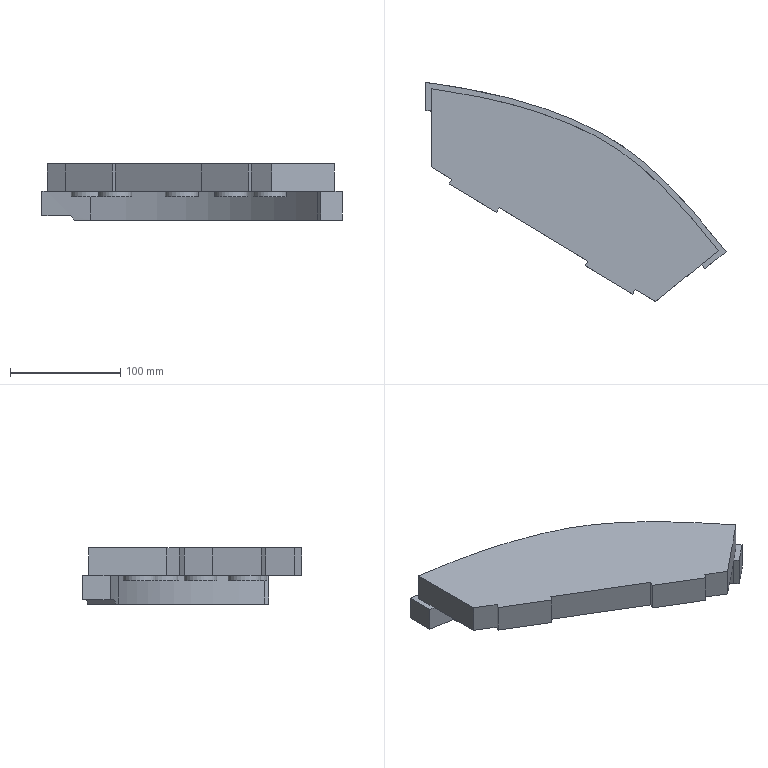Part | NX | features solid 2 | 1 solid | 36 faces | box 271.95 x 198.601 x 51 mm | volume 834371 mm3 | plane 25 | spline 6 | cylinder 5 | commonest cylinder face diameters 30 x5
STEP:
#1=CARTESIAN_POINT('',(-298.429,-300.345,20.));
#2=VERTEX_POINT('',#1);
#3=CARTESIAN_POINT('',(-283.429,-300.345,20.));
#4=DIRECTION('',(0.,0.,-1.));
#5=DIRECTION('',(-1.,0.,0.));
#6=AXIS2_PLACEMENT_3D('',#3,#4,#5);
#7=CIRCLE('',#6,15.);
#8=EDGE_CURVE('',#2,#2,#7,.T.);
#9=ORIENTED_EDGE('',*,*,#8,.F.);
#10=EDGE_LOOP('',(#9));
#11=FACE_BOUND('',#10,.T.);
#12=CARTESIAN_POINT('',(-213.429,-355.345,20.));
#13=VERTEX_POINT('',#12);
#14=CARTESIAN_POINT('',(-198.429,-355.345,20.));
#15=DIRECTION('',(0.,0.,-1.));
#16=DIRECTION('',(-1.,0.,0.));
#17=AXIS2_PLACEMENT_3D('',#14,#15,#16);
#18=CIRCLE('',#17,15.);
#19=EDGE_CURVE('',#13,#13,#18,.T.);
#20=ORIENTED_EDGE('',*,*,#19,.F.);
#21=EDGE_LOOP('',(#20));
#22=FACE_BOUND('',#21,.T.);
#23=CARTESIAN_POINT('',(-103.429,-400.345,20.));
#24=VERTEX_POINT('',#23);
#25=CARTESIAN_POINT('',(-118.429,-400.345,20.));
#26=DIRECTION('',(0.,0.,1.));
#27=DIRECTION('',(1.,0.,0.));
#28=AXIS2_PLACEMENT_3D('',#25,#26,#27);
#29=CIRCLE('',#28,15.);
#30=EDGE_CURVE('',#24,#24,#29,.T.);
#31=ORIENTED_EDGE('',*,*,#30,.T.);
#32=EDGE_LOOP('',(#31));
#33=FACE_BOUND('',#32,.T.);
#34=CARTESIAN_POINT('',(-320.,-324.952,20.));
#35=VERTEX_POINT('',#34);
#36=CARTESIAN_POINT('',(-320.,-274.295,20.));
#37=VERTEX_POINT('',#36);
#38=CARTESIAN_POINT('',(-320.,-348.688,20.));
#39=DIRECTION('',(0.,1.,0.));
#40=VECTOR('',#39,1000.);
#41=LINE('',#38,#40);
#42=EDGE_CURVE('',#35,#37,#41,.T.);
#43=ORIENTED_EDGE('',*,*,#42,.T.);
#44=CARTESIAN_POINT('',(-280.742,-281.088,20.));
#45=VERTEX_POINT('',#44);
#46=CARTESIAN_POINT('',(-280.742,-281.088,20.));
#47=CARTESIAN_POINT('',(-293.762,-278.446,20.));
#48=CARTESIAN_POINT('',(-306.859,-276.24,20.));
#49=CARTESIAN_POINT('',(-320.,-274.295,20.));
#50=B_SPLINE_CURVE_WITH_KNOTS('',3,(#46,#47,#48,#49),.UNSPECIFIED.,.F.,.F.,(4,4),(1.18,1.219),.UNSPECIFIED.);
#51=EDGE_CURVE('',#45,#37,#50,.T.);
#52=ORIENTED_EDGE('',*,*,#51,.F.);
#53=CARTESIAN_POINT('',(-280.742,-281.088,20.));
#54=VERTEX_POINT('',#53);
#55=CARTESIAN_POINT('',(-303.787,-389.506,20.));
#56=DIRECTION('',(-0.2079,-0.9781,0.));
#57=VECTOR('',#56,1000.);
#58=LINE('',#55,#57);
#59=EDGE_CURVE('',#45,#54,#58,.F.);
#60=ORIENTED_EDGE('',*,*,#59,.T.);
#61=CARTESIAN_POINT('',(-75.598,-413.386,20.));
#62=VERTEX_POINT('',#61);
#63=CARTESIAN_POINT('',(-280.742,-281.088,20.));
#64=CARTESIAN_POINT('',(-270.509,-283.168,20.));
#65=CARTESIAN_POINT('',(-250.227,-287.836,20.));
#66=CARTESIAN_POINT('',(-225.511,-295.448,20.));
#67=CARTESIAN_POINT('',(-206.19,-302.794,20.));
#68=CARTESIAN_POINT('',(-191.924,-308.939,20.));
#69=CARTESIAN_POINT('',(-177.971,-315.925,20.));
#70=CARTESIAN_POINT('',(-164.415,-324.129,20.));
#71=CARTESIAN_POINT('',(-151.409,-333.446,20.));
#72=CARTESIAN_POINT('',(-135.17,-346.814,20.));
#73=CARTESIAN_POINT('',(-116.381,-365.121,20.));
#74=CARTESIAN_POINT('',(-95.487,-388.742,20.));
#75=CARTESIAN_POINT('',(-82.188,-405.145,20.));
#76=CARTESIAN_POINT('',(-75.598,-413.386,20.));
#77=B_SPLINE_CURVE_WITH_KNOTS('',3,(#63,#64,#65,#66,#67,#68,#69,#70,#71,#72,#73,#74,#75,#76),.UNSPECIFIED.,.F.,.F.,(4,1,1,1,1,1,1,1,1,1,1,4),(0.9834,1.015,1.046,1.062,1.077,1.093,1.109,1.124,1.14,1.171,1.203,1.234),.UNSPECIFIED.);
#78=EDGE_CURVE('',#62,#54,#77,.F.);
#79=ORIENTED_EDGE('',*,*,#78,.F.);
#80=CARTESIAN_POINT('',(-117.01,-446.921,20.));
#81=VERTEX_POINT('',#80);
#82=CARTESIAN_POINT('',(-152.811,-475.913,20.));
#83=DIRECTION('',(0.7771,0.6293,0.));
#84=VECTOR('',#83,1000.);
#85=LINE('',#82,#84);
#86=EDGE_CURVE('',#81,#62,#85,.T.);
#87=ORIENTED_EDGE('',*,*,#86,.F.);
#88=CARTESIAN_POINT('',(-135.335,-435.91,20.));
#89=VERTEX_POINT('',#88);
#90=CARTESIAN_POINT('',(-344.41,-310.285,20.));
#91=DIRECTION('',(-0.8572,0.515,0.));
#92=VECTOR('',#91,1000.);
#93=LINE('',#90,#92);
#94=EDGE_CURVE('',#89,#81,#93,.F.);
#95=ORIENTED_EDGE('',*,*,#94,.F.);
#96=CARTESIAN_POINT('',(-137.91,-440.196,20.));
#97=VERTEX_POINT('',#96);
#98=CARTESIAN_POINT('',(-135.335,-435.91,20.));
#99=DIRECTION('',(-0.515,-0.8572,0.));
#100=VECTOR('',#99,1000.);
#101=LINE('',#98,#100);
#102=EDGE_CURVE('',#89,#97,#101,.T.);
#103=ORIENTED_EDGE('',*,*,#102,.T.);
#104=CARTESIAN_POINT('',(-180.768,-414.444,20.));
#105=VERTEX_POINT('',#104);
#106=CARTESIAN_POINT('',(-185.054,-411.869,20.));
#107=DIRECTION('',(0.8572,-0.515,0.));
#108=VECTOR('',#107,1000.);
#109=LINE('',#106,#108);
#110=EDGE_CURVE('',#105,#97,#109,.T.);
#111=ORIENTED_EDGE('',*,*,#110,.F.);
#112=CARTESIAN_POINT('',(-178.193,-410.158,20.));
#113=VERTEX_POINT('',#112);
#114=CARTESIAN_POINT('',(-178.193,-410.158,20.));
#115=DIRECTION('',(-0.515,-0.8572,0.));
#116=VECTOR('',#115,1000.);
#117=LINE('',#114,#116);
#118=EDGE_CURVE('',#113,#105,#117,.T.);
#119=ORIENTED_EDGE('',*,*,#118,.F.);
#120=CARTESIAN_POINT('',(-258.498,-361.906,20.));
#121=VERTEX_POINT('',#120);
#122=CARTESIAN_POINT('',(-344.41,-310.285,20.));
#123=DIRECTION('',(-0.8572,0.515,0.));
#124=VECTOR('',#123,1000.);
#125=LINE('',#122,#124);
#126=EDGE_CURVE('',#121,#113,#125,.F.);
#127=ORIENTED_EDGE('',*,*,#126,.F.);
#128=CARTESIAN_POINT('',(-261.073,-366.192,20.));
#129=VERTEX_POINT('',#128);
#130=CARTESIAN_POINT('',(-221.506,-300.342,20.));
#131=DIRECTION('',(0.515,0.8572,0.));
#132=VECTOR('',#131,1000.);
#133=LINE('',#130,#132);
#134=EDGE_CURVE('',#121,#129,#133,.F.);
#135=ORIENTED_EDGE('',*,*,#134,.T.);
#136=CARTESIAN_POINT('',(-303.932,-340.44,20.));
#137=VERTEX_POINT('',#136);
#138=CARTESIAN_POINT('',(-286.788,-350.741,20.));
#139=DIRECTION('',(0.8572,-0.515,0.));
#140=VECTOR('',#139,1000.);
#141=LINE('',#138,#140);
#142=EDGE_CURVE('',#137,#129,#141,.T.);
#143=ORIENTED_EDGE('',*,*,#142,.F.);
#144=CARTESIAN_POINT('',(-301.356,-336.154,20.));
#145=VERTEX_POINT('',#144);
#146=CARTESIAN_POINT('',(-264.365,-274.59,20.));
#147=DIRECTION('',(0.515,0.8572,0.));
#148=VECTOR('',#147,1000.);
#149=LINE('',#146,#148);
#150=EDGE_CURVE('',#145,#137,#149,.F.);
#151=ORIENTED_EDGE('',*,*,#150,.F.);
#152=CARTESIAN_POINT('',(-344.41,-310.285,20.));
#153=DIRECTION('',(-0.8572,0.515,0.));
#154=VECTOR('',#153,1000.);
#155=LINE('',#152,#154);
#156=EDGE_CURVE('',#35,#145,#155,.F.);
#157=ORIENTED_EDGE('',*,*,#156,.F.);
#158=EDGE_LOOP('',(#43,#52,#60,#79,#87,#95,#103,#111,#119,#127,#135,#143,#151,#157));
#159=FACE_BOUND('',#158,.T.);
#160=CARTESIAN_POINT('',(-273.429,-320.345,20.));
#161=VERTEX_POINT('',#160);
#162=CARTESIAN_POINT('',(-258.429,-320.345,20.));
#163=DIRECTION('',(0.,0.,-1.));
#164=DIRECTION('',(-1.,0.,0.));
#165=AXIS2_PLACEMENT_3D('',#162,#163,#164);
#166=CIRCLE('',#165,15.);
#167=EDGE_CURVE('',#161,#161,#166,.T.);
#168=ORIENTED_EDGE('',*,*,#167,.F.);
#169=EDGE_LOOP('',(#168));
#170=FACE_BOUND('',#169,.T.);
#171=CARTESIAN_POINT('',(-168.429,-395.345,20.));
#172=VERTEX_POINT('',#171);
#173=CARTESIAN_POINT('',(-153.429,-395.345,20.));
#174=DIRECTION('',(0.,0.,-1.));
#175=DIRECTION('',(-1.,0.,0.));
#176=AXIS2_PLACEMENT_3D('',#173,#174,#175);
#177=CIRCLE('',#176,15.);
#178=EDGE_CURVE('',#172,#172,#177,.T.);
#179=ORIENTED_EDGE('',*,*,#178,.F.);
#180=EDGE_LOOP('',(#179));
#181=FACE_BOUND('',#180,.T.);
#182=CARTESIAN_POINT('',(-53.05,-401.561,20.));
#183=DIRECTION('',(0.,0.,-1.));
#184=DIRECTION('',(-1.,0.,0.));
#185=AXIS2_PLACEMENT_3D('',#182,#183,#184);
#186=PLANE('',#185);
#187=ADVANCED_FACE('',(#11,#22,#33,#159,#170,#181),#186,.T.);
#188=CARTESIAN_POINT('',(-325.,-273.568,-2.));
#189=VERTEX_POINT('',#188);
#190=CARTESIAN_POINT('',(-325.,-248.32,-2.));
#191=VERTEX_POINT('',#190);
#192=CARTESIAN_POINT('',(-325.,-560.,-2.));
#193=DIRECTION('',(0.,1.,0.));
#194=VECTOR('',#193,1000.);
#195=LINE('',#192,#194);
#196=EDGE_CURVE('',#189,#191,#195,.T.);
#197=ORIENTED_EDGE('',*,*,#196,.F.);
#198=CARTESIAN_POINT('',(-325.,-273.568,20.));
#199=VERTEX_POINT('',#198);
#200=CARTESIAN_POINT('',(-325.,-273.568,7.));
#201=DIRECTION('',(0.,0.,1.));
#202=VECTOR('',#201,1000.);
#203=LINE('',#200,#202);
#204=EDGE_CURVE('',#199,#189,#203,.F.);
#205=ORIENTED_EDGE('',*,*,#204,.F.);
#206=CARTESIAN_POINT('',(-325.,-248.32,20.));
#207=VERTEX_POINT('',#206);
#208=CARTESIAN_POINT('',(-325.,-401.561,20.));
#209=DIRECTION('',(0.,1.,0.));
#210=VECTOR('',#209,1000.);
#211=LINE('',#208,#210);
#212=EDGE_CURVE('',#207,#199,#211,.F.);
#213=ORIENTED_EDGE('',*,*,#212,.F.);
#214=CARTESIAN_POINT('',(-325.,-248.32,7.));
#215=DIRECTION('',(0.,0.,-1.));
#216=VECTOR('',#215,1000.);
#217=LINE('',#214,#216);
#218=EDGE_CURVE('',#191,#207,#217,.F.);
#219=ORIENTED_EDGE('',*,*,#218,.F.);
#220=EDGE_LOOP('',(#197,#205,#213,#219));
#221=FACE_BOUND('',#220,.T.);
#222=CARTESIAN_POINT('',(-325.,-560.,0.));
#223=DIRECTION('',(1.,0.,0.));
#224=DIRECTION('',(0.,0.,-1.));
#225=AXIS2_PLACEMENT_3D('',#222,#223,#224);
#226=PLANE('',#225);
#227=ADVANCED_FACE('',(#221),#226,.F.);
#228=CARTESIAN_POINT('',(-320.,-324.952,45.));
#229=VERTEX_POINT('',#228);
#230=CARTESIAN_POINT('',(-320.,-324.952,70.));
#231=DIRECTION('',(0.,0.,1.));
#232=VECTOR('',#231,1000.);
#233=LINE('',#230,#232);
#234=EDGE_CURVE('',#35,#229,#233,.T.);
#235=ORIENTED_EDGE('',*,*,#234,.F.);
#236=ORIENTED_EDGE('',*,*,#156,.T.);
#237=CARTESIAN_POINT('',(-301.356,-336.154,45.));
#238=VERTEX_POINT('',#237);
#239=CARTESIAN_POINT('',(-301.356,-336.154,45.));
#240=DIRECTION('',(0.,0.,-1.));
#241=VECTOR('',#240,1000.);
#242=LINE('',#239,#241);
#243=EDGE_CURVE('',#238,#145,#242,.T.);
#244=ORIENTED_EDGE('',*,*,#243,.F.);
#245=CARTESIAN_POINT('',(-344.41,-310.285,45.));
#246=DIRECTION('',(0.8572,-0.515,0.));
#247=VECTOR('',#246,1000.);
#248=LINE('',#245,#247);
#249=EDGE_CURVE('',#229,#238,#248,.T.);
#250=ORIENTED_EDGE('',*,*,#249,.F.);
#251=EDGE_LOOP('',(#235,#236,#244,#250));
#252=FACE_BOUND('',#251,.T.);
#253=CARTESIAN_POINT('',(-344.41,-310.285,70.));
#254=DIRECTION('',(0.515,0.8572,0.));
#255=DIRECTION('',(-0.8572,0.515,0.));
#256=AXIS2_PLACEMENT_3D('',#253,#254,#255);
#257=PLANE('',#256);
#258=ADVANCED_FACE('',(#252),#257,.F.);
#259=CARTESIAN_POINT('',(-320.,-254.082,45.));
#260=VERTEX_POINT('',#259);
#261=CARTESIAN_POINT('',(-320.,-254.082,20.));
#262=VERTEX_POINT('',#261);
#263=CARTESIAN_POINT('',(-320.,-254.082,32.5));
#264=DIRECTION('',(0.,0.,-1.));
#265=VECTOR('',#264,1000.);
#266=LINE('',#263,#265);
#267=EDGE_CURVE('',#260,#262,#266,.T.);
#268=ORIENTED_EDGE('',*,*,#267,.F.);
#269=CARTESIAN_POINT('',(-276.584,-261.524,45.));
#270=VERTEX_POINT('',#269);
#271=CARTESIAN_POINT('',(-276.584,-261.524,45.));
#272=CARTESIAN_POINT('',(-290.986,-258.597,45.));
#273=CARTESIAN_POINT('',(-305.47,-256.189,45.));
#274=CARTESIAN_POINT('',(-320.,-254.082,45.));
#275=B_SPLINE_CURVE_WITH_KNOTS('',3,(#271,#272,#273,#274),.UNSPECIFIED.,.F.,.F.,(4,4),(0.,0.04404),.UNSPECIFIED.);
#276=EDGE_CURVE('',#270,#260,#275,.T.);
#277=ORIENTED_EDGE('',*,*,#276,.F.);
#278=CARTESIAN_POINT('',(-276.584,-261.524,20.));
#279=VERTEX_POINT('',#278);
#280=CARTESIAN_POINT('',(-276.584,-261.524,32.5));
#281=DIRECTION('',(0.,0.,-1.));
#282=VECTOR('',#281,1000.);
#283=LINE('',#280,#282);
#284=EDGE_CURVE('',#270,#279,#283,.T.);
#285=ORIENTED_EDGE('',*,*,#284,.T.);
#286=CARTESIAN_POINT('',(-276.584,-261.524,20.));
#287=CARTESIAN_POINT('',(-290.982,-258.598,20.));
#288=CARTESIAN_POINT('',(-305.477,-256.188,20.));
#289=CARTESIAN_POINT('',(-320.,-254.082,20.));
#290=B_SPLINE_CURVE_WITH_KNOTS('',3,(#286,#287,#288,#289),.UNSPECIFIED.,.F.,.F.,(4,4),(1.179,1.223),.UNSPECIFIED.);
#291=EDGE_CURVE('',#279,#262,#290,.T.);
#292=ORIENTED_EDGE('',*,*,#291,.T.);
#293=EDGE_LOOP('',(#268,#277,#285,#292));
#294=FACE_BOUND('',#293,.T.);
#295=CARTESIAN_POINT('',(-276.584,-261.524,45.));
#296=CARTESIAN_POINT('',(-276.584,-261.524,20.));
#297=CARTESIAN_POINT('',(-290.952,-258.604,45.));
#298=CARTESIAN_POINT('',(-290.952,-258.604,20.));
#299=CARTESIAN_POINT('',(-305.447,-256.192,45.));
#300=CARTESIAN_POINT('',(-305.447,-256.192,20.));
#301=CARTESIAN_POINT('',(-320.,-254.082,45.));
#302=CARTESIAN_POINT('',(-320.,-254.082,20.));
#303=B_SPLINE_SURFACE_WITH_KNOTS('',3,1,((#295,#296),(#297,#298),(#299,#300),(#301,#302)),.SURF_OF_LINEAR_EXTRUSION.,.F.,.F.,.F.,(4,4),(2,2),(0.0001519,0.1506),(0.,1.),.PIECEWISE_BEZIER_KNOTS.);
#304=ADVANCED_FACE('',(#294),#303,.F.);
#305=ORIENTED_EDGE('',*,*,#276,.T.);
#306=CARTESIAN_POINT('',(-320.,-348.688,45.));
#307=DIRECTION('',(0.,1.,0.));
#308=VECTOR('',#307,1000.);
#309=LINE('',#306,#308);
#310=EDGE_CURVE('',#229,#260,#309,.T.);
#311=ORIENTED_EDGE('',*,*,#310,.F.);
#312=ORIENTED_EDGE('',*,*,#249,.T.);
#313=CARTESIAN_POINT('',(-303.932,-340.44,45.));
#314=VERTEX_POINT('',#313);
#315=CARTESIAN_POINT('',(-692.191,-986.612,45.));
#316=DIRECTION('',(-0.515,-0.8572,0.));
#317=VECTOR('',#316,1000.);
#318=LINE('',#315,#317);
#319=EDGE_CURVE('',#238,#314,#318,.T.);
#320=ORIENTED_EDGE('',*,*,#319,.T.);
#321=CARTESIAN_POINT('',(-261.073,-366.192,45.));
#322=VERTEX_POINT('',#321);
#323=CARTESIAN_POINT('',(-286.788,-350.741,45.));
#324=DIRECTION('',(0.8572,-0.515,0.));
#325=VECTOR('',#324,1000.);
#326=LINE('',#323,#325);
#327=EDGE_CURVE('',#314,#322,#326,.T.);
#328=ORIENTED_EDGE('',*,*,#327,.T.);
#329=CARTESIAN_POINT('',(-258.498,-361.906,45.));
#330=VERTEX_POINT('',#329);
#331=CARTESIAN_POINT('',(-649.332,-1012.364,45.));
#332=DIRECTION('',(-0.515,-0.8572,0.));
#333=VECTOR('',#332,1000.);
#334=LINE('',#331,#333);
#335=EDGE_CURVE('',#330,#322,#334,.T.);
#336=ORIENTED_EDGE('',*,*,#335,.F.);
#337=CARTESIAN_POINT('',(-178.193,-410.158,45.));
#338=VERTEX_POINT('',#337);
#339=CARTESIAN_POINT('',(-344.41,-310.285,45.));
#340=DIRECTION('',(0.8572,-0.515,0.));
#341=VECTOR('',#340,1000.);
#342=LINE('',#339,#341);
#343=EDGE_CURVE('',#330,#338,#342,.T.);
#344=ORIENTED_EDGE('',*,*,#343,.T.);
#345=CARTESIAN_POINT('',(-180.768,-414.444,45.));
#346=VERTEX_POINT('',#345);
#347=CARTESIAN_POINT('',(-178.193,-410.158,45.));
#348=DIRECTION('',(-0.515,-0.8572,0.));
#349=VECTOR('',#348,1000.);
#350=LINE('',#347,#349);
#351=EDGE_CURVE('',#338,#346,#350,.T.);
#352=ORIENTED_EDGE('',*,*,#351,.T.);
#353=CARTESIAN_POINT('',(-137.91,-440.196,45.));
#354=VERTEX_POINT('',#353);
#355=CARTESIAN_POINT('',(-185.054,-411.869,45.));
#356=DIRECTION('',(0.8572,-0.515,0.));
#357=VECTOR('',#356,1000.);
#358=LINE('',#355,#357);
#359=EDGE_CURVE('',#346,#354,#358,.T.);
#360=ORIENTED_EDGE('',*,*,#359,.T.);
#361=CARTESIAN_POINT('',(-135.335,-435.91,45.));
#362=VERTEX_POINT('',#361);
#363=CARTESIAN_POINT('',(-135.335,-435.91,45.));
#364=DIRECTION('',(-0.515,-0.8572,0.));
#365=VECTOR('',#364,1000.);
#366=LINE('',#363,#365);
#367=EDGE_CURVE('',#362,#354,#366,.T.);
#368=ORIENTED_EDGE('',*,*,#367,.F.);
#369=CARTESIAN_POINT('',(-117.01,-446.921,45.));
#370=VERTEX_POINT('',#369);
#371=CARTESIAN_POINT('',(-344.41,-310.285,45.));
#372=DIRECTION('',(0.8572,-0.515,0.));
#373=VECTOR('',#372,1000.);
#374=LINE('',#371,#373);
#375=EDGE_CURVE('',#362,#370,#374,.T.);
#376=ORIENTED_EDGE('',*,*,#375,.T.);
#377=CARTESIAN_POINT('',(-60.055,-400.8,45.));
#378=VERTEX_POINT('',#377);
#379=CARTESIAN_POINT('',(-152.811,-475.913,45.));
#380=DIRECTION('',(-0.7771,-0.6293,0.));
#381=VECTOR('',#380,1000.);
#382=LINE('',#379,#381);
#383=EDGE_CURVE('',#370,#378,#382,.F.);
#384=ORIENTED_EDGE('',*,*,#383,.T.);
#385=CARTESIAN_POINT('',(-60.055,-400.8,45.));
#386=CARTESIAN_POINT('',(-66.959,-392.166,45.));
#387=CARTESIAN_POINT('',(-80.881,-375.009,45.));
#388=CARTESIAN_POINT('',(-102.927,-350.204,45.));
#389=CARTESIAN_POINT('',(-126.762,-327.198,45.));
#390=CARTESIAN_POINT('',(-148.381,-310.537,45.));
#391=CARTESIAN_POINT('',(-167.072,-299.096,45.));
#392=CARTESIAN_POINT('',(-181.889,-291.536,45.));
#393=CARTESIAN_POINT('',(-197.172,-284.86,45.));
#394=CARTESIAN_POINT('',(-217.794,-276.927,45.));
#395=CARTESIAN_POINT('',(-244.14,-268.728,45.));
#396=CARTESIAN_POINT('',(-265.708,-263.735,45.));
#397=CARTESIAN_POINT('',(-276.584,-261.524,45.));
#398=B_SPLINE_CURVE_WITH_KNOTS('',3,(#385,#386,#387,#388,#389,#390,#391,#392,#393,#394,#395,#396,#397),.UNSPECIFIED.,.F.,.F.,(4,1,1,1,1,1,1,1,1,1,4),(0.,0.03314,0.06628,0.09942,0.1326,0.1491,0.1657,0.1823,0.1988,0.232,0.2651),.UNSPECIFIED.);
#399=EDGE_CURVE('',#378,#270,#398,.T.);
#400=ORIENTED_EDGE('',*,*,#399,.T.);
#401=EDGE_LOOP('',(#305,#311,#312,#320,#328,#336,#344,#352,#360,#368,#376,#384,#400));
#402=FACE_BOUND('',#401,.T.);
#403=CARTESIAN_POINT('',(-582.311,-1052.635,45.));
#404=DIRECTION('',(0.,0.,1.));
#405=DIRECTION('',(1.,0.,0.));
#406=AXIS2_PLACEMENT_3D('',#403,#404,#405);
#407=PLANE('',#406);
#408=ADVANCED_FACE('',(#402),#407,.T.);
#409=CARTESIAN_POINT('',(-103.429,-400.345,15.));
#410=VERTEX_POINT('',#409);
#411=CARTESIAN_POINT('',(-118.429,-400.345,15.));
#412=DIRECTION('',(0.,0.,1.));
#413=DIRECTION('',(1.,0.,0.));
#414=AXIS2_PLACEMENT_3D('',#411,#412,#413);
#415=CIRCLE('',#414,15.);
#416=EDGE_CURVE('',#410,#410,#415,.T.);
#417=ORIENTED_EDGE('',*,*,#416,.F.);
#418=EDGE_LOOP('',(#417));
#419=FACE_BOUND('',#418,.T.);
#420=CARTESIAN_POINT('',(-118.429,-400.345,15.));
#421=DIRECTION('',(0.,0.,1.));
#422=DIRECTION('',(1.,0.,0.));
#423=AXIS2_PLACEMENT_3D('',#420,#421,#422);
#424=PLANE('',#423);
#425=ADVANCED_FACE('',(#419),#424,.F.);
#426=CARTESIAN_POINT('',(-53.05,-401.561,20.));
#427=VERTEX_POINT('',#426);
#428=CARTESIAN_POINT('',(-72.479,-417.295,20.));
#429=VERTEX_POINT('',#428);
#430=CARTESIAN_POINT('',(-1582.481,-1640.07,20.));
#431=DIRECTION('',(0.7771,0.6293,0.));
#432=VECTOR('',#431,1000.);
#433=LINE('',#430,#432);
#434=EDGE_CURVE('',#427,#429,#433,.F.);
#435=ORIENTED_EDGE('',*,*,#434,.T.);
#436=CARTESIAN_POINT('',(-72.479,-417.295,-6.));
#437=VERTEX_POINT('',#436);
#438=CARTESIAN_POINT('',(-72.479,-417.295,9.5));
#439=DIRECTION('',(0.,0.,1.));
#440=VECTOR('',#439,1000.);
#441=LINE('',#438,#440);
#442=EDGE_CURVE('',#429,#437,#441,.F.);
#443=ORIENTED_EDGE('',*,*,#442,.T.);
#444=CARTESIAN_POINT('',(-53.05,-401.561,-6.));
#445=VERTEX_POINT('',#444);
#446=CARTESIAN_POINT('',(-1582.481,-1640.07,-6.));
#447=DIRECTION('',(0.7771,0.6293,0.));
#448=VECTOR('',#447,1000.);
#449=LINE('',#446,#448);
#450=EDGE_CURVE('',#437,#445,#449,.T.);
#451=ORIENTED_EDGE('',*,*,#450,.T.);
#452=CARTESIAN_POINT('',(-53.05,-401.561,70.));
#453=DIRECTION('',(0.,0.,-1.));
#454=VECTOR('',#453,1000.);
#455=LINE('',#452,#454);
#456=EDGE_CURVE('',#427,#445,#455,.T.);
#457=ORIENTED_EDGE('',*,*,#456,.F.);
#458=EDGE_LOOP('',(#435,#443,#451,#457));
#459=FACE_BOUND('',#458,.T.);
#460=CARTESIAN_POINT('',(-1582.481,-1640.07,70.));
#461=DIRECTION('',(-0.6293,0.7771,0.));
#462=DIRECTION('',(-0.7771,-0.6293,0.));
#463=AXIS2_PLACEMENT_3D('',#460,#461,#462);
#464=PLANE('',#463);
#465=ADVANCED_FACE('',(#459),#464,.F.);
#466=CARTESIAN_POINT('',(-75.54,-413.459,20.));
#467=VERTEX_POINT('',#466);
#468=CARTESIAN_POINT('',(-75.54,-413.459,20.));
#469=CARTESIAN_POINT('',(-74.518,-414.736,20.));
#470=CARTESIAN_POINT('',(-73.498,-416.015,20.));
#471=CARTESIAN_POINT('',(-72.479,-417.295,20.));
#472=B_SPLINE_CURVE_WITH_KNOTS('',3,(#468,#469,#470,#471),.UNSPECIFIED.,.F.,.F.,(4,4),(0.07392,0.07882),.UNSPECIFIED.);
#473=EDGE_CURVE('',#467,#429,#472,.T.);
#474=ORIENTED_EDGE('',*,*,#473,.F.);
#475=CARTESIAN_POINT('',(-75.54,-413.459,-6.));
#476=VERTEX_POINT('',#475);
#477=CARTESIAN_POINT('',(-75.54,-413.459,-10.));
#478=DIRECTION('',(0.,0.,1.));
#479=VECTOR('',#478,1000.);
#480=LINE('',#477,#479);
#481=EDGE_CURVE('',#467,#476,#480,.F.);
#482=ORIENTED_EDGE('',*,*,#481,.T.);
#483=CARTESIAN_POINT('',(-72.479,-417.295,-6.));
#484=CARTESIAN_POINT('',(-73.498,-416.015,-6.));
#485=CARTESIAN_POINT('',(-74.518,-414.736,-6.));
#486=CARTESIAN_POINT('',(-75.54,-413.459,-6.));
#487=B_SPLINE_CURVE_WITH_KNOTS('',3,(#483,#484,#485,#486),.UNSPECIFIED.,.F.,.F.,(4,4),(0.0276,0.0325),.UNSPECIFIED.);
#488=EDGE_CURVE('',#437,#476,#487,.T.);
#489=ORIENTED_EDGE('',*,*,#488,.F.);
#490=ORIENTED_EDGE('',*,*,#442,.F.);
#491=EDGE_LOOP('',(#474,#482,#489,#490));
#492=FACE_BOUND('',#491,.T.);
#493=CARTESIAN_POINT('',(-72.479,-417.295,-6.));
#494=CARTESIAN_POINT('',(-72.479,-417.295,20.));
#495=CARTESIAN_POINT('',(-73.507,-416.003,-6.));
#496=CARTESIAN_POINT('',(-73.507,-416.003,20.));
#497=CARTESIAN_POINT('',(-74.52,-414.734,-6.));
#498=CARTESIAN_POINT('',(-74.52,-414.734,20.));
#499=CARTESIAN_POINT('',(-75.54,-413.459,-6.));
#500=CARTESIAN_POINT('',(-75.54,-413.459,20.));
#501=B_SPLINE_SURFACE_WITH_KNOTS('',3,1,((#493,#494),(#495,#496),(#497,#498),(#499,#500)),.SURF_OF_LINEAR_EXTRUSION.,.F.,.F.,.F.,(4,4),(2,2),(-0.0007285,0.0174),(0.,1.),.PIECEWISE_BEZIER_KNOTS.);
#502=ADVANCED_FACE('',(#492),#501,.F.);
#503=CARTESIAN_POINT('',(-303.932,-340.44,45.));
#504=DIRECTION('',(0.,0.,-1.));
#505=VECTOR('',#504,1000.);
#506=LINE('',#503,#505);
#507=EDGE_CURVE('',#314,#137,#506,.T.);
#508=ORIENTED_EDGE('',*,*,#507,.F.);
#509=ORIENTED_EDGE('',*,*,#319,.F.);
#510=ORIENTED_EDGE('',*,*,#243,.T.);
#511=ORIENTED_EDGE('',*,*,#150,.T.);
#512=EDGE_LOOP('',(#508,#509,#510,#511));
#513=FACE_BOUND('',#512,.T.);
#514=CARTESIAN_POINT('',(-301.356,-336.154,45.));
#515=DIRECTION('',(-0.8572,0.515,0.));
#516=DIRECTION('',(-0.515,-0.8572,0.));
#517=AXIS2_PLACEMENT_3D('',#514,#515,#516);
#518=PLANE('',#517);
#519=ADVANCED_FACE('',(#513),#518,.T.);
#520=CARTESIAN_POINT('',(-261.073,-366.192,45.));
#521=DIRECTION('',(0.,0.,-1.));
#522=VECTOR('',#521,1000.);
#523=LINE('',#520,#522);
#524=EDGE_CURVE('',#322,#129,#523,.T.);
#525=ORIENTED_EDGE('',*,*,#524,.F.);
#526=ORIENTED_EDGE('',*,*,#327,.F.);
#527=ORIENTED_EDGE('',*,*,#507,.T.);
#528=ORIENTED_EDGE('',*,*,#142,.T.);
#529=EDGE_LOOP('',(#525,#526,#527,#528));
#530=FACE_BOUND('',#529,.T.);
#531=CARTESIAN_POINT('',(-286.788,-350.741,45.));
#532=DIRECTION('',(-0.515,-0.8572,0.));
#533=DIRECTION('',(0.,0.,-1.));
#534=AXIS2_PLACEMENT_3D('',#531,#532,#533);
#535=PLANE('',#534);
#536=ADVANCED_FACE('',(#530),#535,.T.);
#537=ORIENTED_EDGE('',*,*,#524,.T.);
#538=ORIENTED_EDGE('',*,*,#134,.F.);
#539=CARTESIAN_POINT('',(-258.498,-361.906,45.));
#540=DIRECTION('',(0.,0.,-1.));
#541=VECTOR('',#540,1000.);
#542=LINE('',#539,#541);
#543=EDGE_CURVE('',#330,#121,#542,.T.);
#544=ORIENTED_EDGE('',*,*,#543,.F.);
#545=ORIENTED_EDGE('',*,*,#335,.T.);
#546=EDGE_LOOP('',(#537,#538,#544,#545));
#547=FACE_BOUND('',#546,.T.);
#548=CARTESIAN_POINT('',(-258.498,-361.906,45.));
#549=DIRECTION('',(-0.8572,0.515,0.));
#550=DIRECTION('',(-0.515,-0.8572,0.));
#551=AXIS2_PLACEMENT_3D('',#548,#549,#550);
#552=PLANE('',#551);
#553=ADVANCED_FACE('',(#547),#552,.F.);
#554=ORIENTED_EDGE('',*,*,#126,.T.);
#555=CARTESIAN_POINT('',(-178.193,-410.158,45.));
#556=DIRECTION('',(0.,0.,1.));
#557=VECTOR('',#556,1000.);
#558=LINE('',#555,#557);
#559=EDGE_CURVE('',#338,#113,#558,.F.);
#560=ORIENTED_EDGE('',*,*,#559,.F.);
#561=ORIENTED_EDGE('',*,*,#343,.F.);
#562=ORIENTED_EDGE('',*,*,#543,.T.);
#563=EDGE_LOOP('',(#554,#560,#561,#562));
#564=FACE_BOUND('',#563,.T.);
#565=CARTESIAN_POINT('',(-344.41,-310.285,70.));
#566=DIRECTION('',(0.515,0.8572,0.));
#567=DIRECTION('',(-0.8572,0.515,0.));
#568=AXIS2_PLACEMENT_3D('',#565,#566,#567);
#569=PLANE('',#568);
#570=ADVANCED_FACE('',(#564),#569,.F.);
#571=CARTESIAN_POINT('',(-180.768,-414.444,45.));
#572=DIRECTION('',(0.,0.,1.));
#573=VECTOR('',#572,1000.);
#574=LINE('',#571,#573);
#575=EDGE_CURVE('',#346,#105,#574,.F.);
#576=ORIENTED_EDGE('',*,*,#575,.F.);
#577=ORIENTED_EDGE('',*,*,#351,.F.);
#578=ORIENTED_EDGE('',*,*,#559,.T.);
#579=ORIENTED_EDGE('',*,*,#118,.T.);
#580=EDGE_LOOP('',(#576,#577,#578,#579));
#581=FACE_BOUND('',#580,.T.);
#582=CARTESIAN_POINT('',(-178.193,-410.158,45.));
#583=DIRECTION('',(-0.8572,0.515,0.));
#584=DIRECTION('',(-0.515,-0.8572,0.));
#585=AXIS2_PLACEMENT_3D('',#582,#583,#584);
#586=PLANE('',#585);
#587=ADVANCED_FACE('',(#581),#586,.T.);
#588=CARTESIAN_POINT('',(-137.91,-440.196,45.));
#589=DIRECTION('',(0.,0.,-1.));
#590=VECTOR('',#589,1000.);
#591=LINE('',#588,#590);
#592=EDGE_CURVE('',#354,#97,#591,.T.);
#593=ORIENTED_EDGE('',*,*,#592,.F.);
#594=ORIENTED_EDGE('',*,*,#359,.F.);
#595=ORIENTED_EDGE('',*,*,#575,.T.);
#596=ORIENTED_EDGE('',*,*,#110,.T.);
#597=EDGE_LOOP('',(#593,#594,#595,#596));
#598=FACE_BOUND('',#597,.T.);
#599=CARTESIAN_POINT('',(-185.054,-411.869,45.));
#600=DIRECTION('',(-0.515,-0.8572,0.));
#601=DIRECTION('',(0.,0.,-1.));
#602=AXIS2_PLACEMENT_3D('',#599,#600,#601);
#603=PLANE('',#602);
#604=ADVANCED_FACE('',(#598),#603,.T.);
#605=ORIENTED_EDGE('',*,*,#592,.T.);
#606=ORIENTED_EDGE('',*,*,#102,.F.);
#607=CARTESIAN_POINT('',(-135.335,-435.91,45.));
#608=DIRECTION('',(0.,0.,-1.));
#609=VECTOR('',#608,1000.);
#610=LINE('',#607,#609);
#611=EDGE_CURVE('',#362,#89,#610,.T.);
#612=ORIENTED_EDGE('',*,*,#611,.F.);
#613=ORIENTED_EDGE('',*,*,#367,.T.);
#614=EDGE_LOOP('',(#605,#606,#612,#613));
#615=FACE_BOUND('',#614,.T.);
#616=CARTESIAN_POINT('',(-135.335,-435.91,45.));
#617=DIRECTION('',(-0.8572,0.515,0.));
#618=DIRECTION('',(-0.515,-0.8572,0.));
#619=AXIS2_PLACEMENT_3D('',#616,#617,#618);
#620=PLANE('',#619);
#621=ADVANCED_FACE('',(#615),#620,.F.);
#622=ORIENTED_EDGE('',*,*,#611,.T.);
#623=ORIENTED_EDGE('',*,*,#94,.T.);
#624=CARTESIAN_POINT('',(-117.01,-446.921,70.));
#625=DIRECTION('',(0.,0.,1.));
#626=VECTOR('',#625,1000.);
#627=LINE('',#624,#626);
#628=EDGE_CURVE('',#370,#81,#627,.F.);
#629=ORIENTED_EDGE('',*,*,#628,.F.);
#630=ORIENTED_EDGE('',*,*,#375,.F.);
#631=EDGE_LOOP('',(#622,#623,#629,#630));
#632=FACE_BOUND('',#631,.T.);
#633=CARTESIAN_POINT('',(-344.41,-310.285,70.));
#634=DIRECTION('',(0.515,0.8572,0.));
#635=DIRECTION('',(-0.8572,0.515,0.));
#636=AXIS2_PLACEMENT_3D('',#633,#634,#635);
#637=PLANE('',#636);
#638=ADVANCED_FACE('',(#632),#637,.F.);
#639=ORIENTED_EDGE('',*,*,#628,.T.);
#640=ORIENTED_EDGE('',*,*,#86,.T.);
#641=CARTESIAN_POINT('',(-60.055,-400.8,20.));
#642=VERTEX_POINT('',#641);
#643=CARTESIAN_POINT('',(-56.196,-397.675,20.));
#644=DIRECTION('',(0.7771,0.6293,0.));
#645=VECTOR('',#644,1000.);
#646=LINE('',#643,#645);
#647=EDGE_CURVE('',#62,#642,#646,.T.);
#648=ORIENTED_EDGE('',*,*,#647,.T.);
#649=CARTESIAN_POINT('',(-60.055,-400.8,42.5));
#650=DIRECTION('',(0.,0.,-1.));
#651=VECTOR('',#650,1000.);
#652=LINE('',#649,#651);
#653=EDGE_CURVE('',#642,#378,#652,.F.);
#654=ORIENTED_EDGE('',*,*,#653,.T.);
#655=ORIENTED_EDGE('',*,*,#383,.F.);
#656=EDGE_LOOP('',(#639,#640,#648,#654,#655));
#657=FACE_BOUND('',#656,.T.);
#658=CARTESIAN_POINT('',(-152.811,-475.913,70.));
#659=DIRECTION('',(0.6293,-0.7771,0.));
#660=DIRECTION('',(0.7771,0.6293,0.));
#661=AXIS2_PLACEMENT_3D('',#658,#659,#660);
#662=PLANE('',#661);
#663=ADVANCED_FACE('',(#657),#662,.T.);
#664=ORIENTED_EDGE('',*,*,#78,.T.);
#665=CARTESIAN_POINT('',(-280.742,-281.088,-6.));
#666=VERTEX_POINT('',#665);
#667=CARTESIAN_POINT('',(-280.742,-281.088,25.));
#668=DIRECTION('',(0.,0.,1.));
#669=VECTOR('',#668,1000.);
#670=LINE('',#667,#669);
#671=EDGE_CURVE('',#54,#666,#670,.F.);
#672=ORIENTED_EDGE('',*,*,#671,.T.);
#673=CARTESIAN_POINT('',(-280.742,-281.088,-6.));
#674=CARTESIAN_POINT('',(-270.511,-283.167,-6.));
#675=CARTESIAN_POINT('',(-250.227,-287.836,-6.));
#676=CARTESIAN_POINT('',(-225.493,-295.453,-6.));
#677=CARTESIAN_POINT('',(-206.149,-302.81,-6.));
#678=CARTESIAN_POINT('',(-191.859,-308.968,-6.));
#679=CARTESIAN_POINT('',(-177.885,-315.97,-6.));
#680=CARTESIAN_POINT('',(-164.271,-324.225,-6.));
#681=CARTESIAN_POINT('',(-151.31,-333.524,-6.));
#682=CARTESIAN_POINT('',(-135.089,-346.888,-6.));
#683=CARTESIAN_POINT('',(-116.319,-365.188,-6.));
#684=CARTESIAN_POINT('',(-95.428,-388.812,-6.));
#685=CARTESIAN_POINT('',(-82.129,-405.218,-6.));
#686=CARTESIAN_POINT('',(-75.54,-413.459,-6.));
#687=B_SPLINE_CURVE_WITH_KNOTS('',3,(#673,#674,#675,#676,#677,#678,#679,#680,#681,#682,#683,#684,#685,#686),.UNSPECIFIED.,.F.,.F.,(4,1,1,1,1,1,1,1,1,1,1,4),(1.004,1.035,1.066,1.082,1.098,1.113,1.129,1.145,1.16,1.192,1.223,1.254),.UNSPECIFIED.);
#688=EDGE_CURVE('',#476,#666,#687,.F.);
#689=ORIENTED_EDGE('',*,*,#688,.F.);
#690=ORIENTED_EDGE('',*,*,#481,.F.);
#691=CARTESIAN_POINT('',(-75.598,-413.386,20.));
#692=CARTESIAN_POINT('',(-75.579,-413.41,20.));
#693=CARTESIAN_POINT('',(-75.559,-413.435,20.));
#694=CARTESIAN_POINT('',(-75.54,-413.459,20.));
#695=B_SPLINE_CURVE_WITH_KNOTS('',3,(#691,#692,#693,#694),.UNSPECIFIED.,.F.,.F.,(4,4),(0.03007,0.03017),.UNSPECIFIED.);
#696=EDGE_CURVE('',#62,#467,#695,.T.);
#697=ORIENTED_EDGE('',*,*,#696,.F.);
#698=EDGE_LOOP('',(#664,#672,#689,#690,#697));
#699=FACE_BOUND('',#698,.T.);
#700=CARTESIAN_POINT('',(-75.54,-413.459,-6.));
#701=CARTESIAN_POINT('',(-75.54,-413.459,20.));
#702=CARTESIAN_POINT('',(-82.456,-404.809,-6.));
#703=CARTESIAN_POINT('',(-82.456,-404.809,20.));
#704=CARTESIAN_POINT('',(-96.271,-387.787,-6.));
#705=CARTESIAN_POINT('',(-96.271,-387.787,20.));
#706=CARTESIAN_POINT('',(-117.577,-363.852,-6.));
#707=CARTESIAN_POINT('',(-117.577,-363.852,20.));
#708=CARTESIAN_POINT('',(-140.087,-342.157,-6.));
#709=CARTESIAN_POINT('',(-140.087,-342.157,20.));
#710=CARTESIAN_POINT('',(-160.228,-326.708,-6.));
#711=CARTESIAN_POINT('',(-160.228,-326.708,20.));
#712=CARTESIAN_POINT('',(-177.125,-316.416,-6.));
#713=CARTESIAN_POINT('',(-177.125,-316.416,20.));
#714=CARTESIAN_POINT('',(-190.547,-309.582,-6.));
#715=CARTESIAN_POINT('',(-190.547,-309.582,20.));
#716=CARTESIAN_POINT('',(-204.812,-303.351,-6.));
#717=CARTESIAN_POINT('',(-204.812,-303.351,20.));
#718=CARTESIAN_POINT('',(-219.486,-297.71,-6.));
#719=CARTESIAN_POINT('',(-219.486,-297.71,20.));
#720=CARTESIAN_POINT('',(-234.388,-292.708,-6.));
#721=CARTESIAN_POINT('',(-234.388,-292.708,20.));
#722=CARTESIAN_POINT('',(-247.031,-289.039,-6.));
#723=CARTESIAN_POINT('',(-247.031,-289.039,20.));
#724=CARTESIAN_POINT('',(-257.284,-286.367,-6.));
#725=CARTESIAN_POINT('',(-257.284,-286.367,20.));
#726=CARTESIAN_POINT('',(-265.044,-284.487,-6.));
#727=CARTESIAN_POINT('',(-265.044,-284.487,20.));
#728=CARTESIAN_POINT('',(-271.54,-283.022,-6.));
#729=CARTESIAN_POINT('',(-271.54,-283.022,20.));
#730=CARTESIAN_POINT('',(-276.81,-281.895,-6.));
#731=CARTESIAN_POINT('',(-276.81,-281.895,20.));
#732=CARTESIAN_POINT('',(-279.37,-281.366,-6.));
#733=CARTESIAN_POINT('',(-279.37,-281.366,20.));
#734=CARTESIAN_POINT('',(-280.742,-281.088,-6.));
#735=CARTESIAN_POINT('',(-280.742,-281.088,20.));
#736=B_SPLINE_SURFACE_WITH_KNOTS('',3,1,((#700,#701),(#702,#703),(#704,#705),(#706,#707),(#708,#709),(#710,#711),(#712,#713),(#714,#715),(#716,#717),(#718,#719),(#720,#721),(#722,#723),(#724,#725),(#726,#727),(#728,#729),(#730,#731),(#732,#733),(#734,#735)),.SURF_OF_LINEAR_EXTRUSION.,.F.,.F.,.F.,(4,1,1,1,1,1,1,1,1,1,1,1,1,1,1,4),(2,2),(0.0174,0.1403,0.2633,0.3862,0.5091,0.5706,0.632,0.6935,0.755,0.8164,0.8779,0.9086,0.9393,0.9701,0.9854,1.001),(0.,1.),.UNSPECIFIED.);
#737=ADVANCED_FACE('',(#699),#736,.F.);
#738=ORIENTED_EDGE('',*,*,#416,.T.);
#739=EDGE_LOOP('',(#738));
#740=FACE_BOUND('',#739,.T.);
#741=ORIENTED_EDGE('',*,*,#30,.F.);
#742=EDGE_LOOP('',(#741));
#743=FACE_BOUND('',#742,.T.);
#744=CARTESIAN_POINT('',(-118.429,-400.345,15.));
#745=DIRECTION('',(0.,0.,1.));
#746=DIRECTION('',(1.,0.,0.));
#747=AXIS2_PLACEMENT_3D('',#744,#745,#746);
#748=CYLINDRICAL_SURFACE('',#747,15.);
#749=ADVANCED_FACE('',(#740,#743),#748,.T.);
#750=ORIENTED_EDGE('',*,*,#284,.F.);
#751=ORIENTED_EDGE('',*,*,#399,.F.);
#752=ORIENTED_EDGE('',*,*,#653,.F.);
#753=CARTESIAN_POINT('',(-60.055,-400.8,20.));
#754=CARTESIAN_POINT('',(-66.968,-392.156,20.));
#755=CARTESIAN_POINT('',(-80.912,-374.973,20.));
#756=CARTESIAN_POINT('',(-102.877,-350.264,20.));
#757=CARTESIAN_POINT('',(-122.666,-331.141,20.));
#758=CARTESIAN_POINT('',(-139.771,-317.163,20.));
#759=CARTESIAN_POINT('',(-153.446,-307.404,20.));
#760=CARTESIAN_POINT('',(-167.702,-298.745,20.));
#761=CARTESIAN_POINT('',(-182.405,-291.3,20.));
#762=CARTESIAN_POINT('',(-197.471,-284.741,20.));
#763=CARTESIAN_POINT('',(-217.915,-276.89,20.));
#764=CARTESIAN_POINT('',(-244.121,-268.734,20.));
#765=CARTESIAN_POINT('',(-265.727,-263.731,20.));
#766=CARTESIAN_POINT('',(-276.584,-261.524,20.));
#767=B_SPLINE_CURVE_WITH_KNOTS('',3,(#753,#754,#755,#756,#757,#758,#759,#760,#761,#762,#763,#764,#765,#766),.UNSPECIFIED.,.F.,.F.,(4,1,1,1,1,1,1,1,1,1,1,4),(0.6916,0.7249,0.7581,0.7913,0.8079,0.8245,0.8411,0.8577,0.8743,0.8909,0.9241,0.9573),.UNSPECIFIED.);
#768=EDGE_CURVE('',#642,#279,#767,.T.);
#769=ORIENTED_EDGE('',*,*,#768,.T.);
#770=EDGE_LOOP('',(#750,#751,#752,#769));
#771=FACE_BOUND('',#770,.T.);
#772=CARTESIAN_POINT('',(-60.055,-400.8,45.));
#773=CARTESIAN_POINT('',(-60.055,-400.8,20.));
#774=CARTESIAN_POINT('',(-73.99,-383.376,45.));
#775=CARTESIAN_POINT('',(-73.99,-383.376,20.));
#776=CARTESIAN_POINT('',(-95.207,-357.63,45.));
#777=CARTESIAN_POINT('',(-95.207,-357.63,20.));
#778=CARTESIAN_POINT('',(-126.963,-327.016,45.));
#779=CARTESIAN_POINT('',(-126.963,-327.016,20.));
#780=CARTESIAN_POINT('',(-148.753,-310.274,45.));
#781=CARTESIAN_POINT('',(-148.753,-310.274,20.));
#782=CARTESIAN_POINT('',(-167.403,-298.917,45.));
#783=CARTESIAN_POINT('',(-167.403,-298.917,20.));
#784=CARTESIAN_POINT('',(-182.036,-291.471,45.));
#785=CARTESIAN_POINT('',(-182.036,-291.471,20.));
#786=CARTESIAN_POINT('',(-197.188,-284.855,45.));
#787=CARTESIAN_POINT('',(-197.188,-284.855,20.));
#788=CARTESIAN_POINT('',(-217.793,-276.928,45.));
#789=CARTESIAN_POINT('',(-217.793,-276.928,20.));
#790=CARTESIAN_POINT('',(-238.857,-270.37,45.));
#791=CARTESIAN_POINT('',(-238.857,-270.37,20.));
#792=CARTESIAN_POINT('',(-260.342,-264.979,45.));
#793=CARTESIAN_POINT('',(-260.342,-264.979,20.));
#794=CARTESIAN_POINT('',(-271.106,-262.638,45.));
#795=CARTESIAN_POINT('',(-271.106,-262.638,20.));
#796=CARTESIAN_POINT('',(-276.584,-261.524,45.));
#797=CARTESIAN_POINT('',(-276.584,-261.524,20.));
#798=B_SPLINE_SURFACE_WITH_KNOTS('',3,1,((#772,#773),(#774,#775),(#776,#777),(#778,#779),(#780,#781),(#782,#783),(#784,#785),(#786,#787),(#788,#789),(#790,#791),(#792,#793),(#794,#795),(#796,#797)),.SURF_OF_LINEAR_EXTRUSION.,.F.,.F.,.F.,(4,1,1,1,1,1,1,1,1,1,4),(2,2),(0.01819,0.2637,0.3864,0.5092,0.5705,0.6319,0.6933,0.7547,0.8774,0.9388,1.),(0.,1.),.UNSPECIFIED.);
#799=ADVANCED_FACE('',(#771),#798,.F.);
#800=ORIENTED_EDGE('',*,*,#671,.F.);
#801=ORIENTED_EDGE('',*,*,#59,.F.);
#802=CARTESIAN_POINT('',(-280.742,-281.088,-6.));
#803=VERTEX_POINT('',#802);
#804=CARTESIAN_POINT('',(-280.742,-281.088,9.5));
#805=DIRECTION('',(0.,0.,1.));
#806=VECTOR('',#805,1000.);
#807=LINE('',#804,#806);
#808=EDGE_CURVE('',#45,#803,#807,.F.);
#809=ORIENTED_EDGE('',*,*,#808,.T.);
#810=CARTESIAN_POINT('',(-573.499,-1658.401,-6.));
#811=DIRECTION('',(0.2079,0.9781,0.));
#812=VECTOR('',#811,1000.);
#813=LINE('',#810,#812);
#814=EDGE_CURVE('',#803,#666,#813,.T.);
#815=ORIENTED_EDGE('',*,*,#814,.T.);
#816=EDGE_LOOP('',(#800,#801,#809,#815));
#817=FACE_BOUND('',#816,.T.);
#818=CARTESIAN_POINT('',(-573.499,-1658.401,70.));
#819=DIRECTION('',(-0.9781,0.2079,0.));
#820=DIRECTION('',(-0.2079,-0.9781,0.));
#821=AXIS2_PLACEMENT_3D('',#818,#819,#820);
#822=PLANE('',#821);
#823=ADVANCED_FACE('',(#817),#822,.F.);
#824=ORIENTED_EDGE('',*,*,#212,.T.);
#825=CARTESIAN_POINT('',(-320.,-274.295,20.));
#826=CARTESIAN_POINT('',(-321.665,-274.049,20.));
#827=CARTESIAN_POINT('',(-323.331,-273.807,20.));
#828=CARTESIAN_POINT('',(-325.,-273.568,20.));
#829=B_SPLINE_CURVE_WITH_KNOTS('',3,(#825,#826,#827,#828),.UNSPECIFIED.,.F.,.F.,(4,4),(0.1405,0.158),.UNSPECIFIED.);
#830=EDGE_CURVE('',#37,#199,#829,.T.);
#831=ORIENTED_EDGE('',*,*,#830,.F.);
#832=CARTESIAN_POINT('',(-320.,-348.688,20.));
#833=DIRECTION('',(0.,1.,0.));
#834=VECTOR('',#833,1000.);
#835=LINE('',#832,#834);
#836=EDGE_CURVE('',#37,#262,#835,.T.);
#837=ORIENTED_EDGE('',*,*,#836,.T.);
#838=ORIENTED_EDGE('',*,*,#291,.F.);
#839=ORIENTED_EDGE('',*,*,#768,.F.);
#840=ORIENTED_EDGE('',*,*,#647,.F.);
#841=ORIENTED_EDGE('',*,*,#696,.T.);
#842=ORIENTED_EDGE('',*,*,#473,.T.);
#843=ORIENTED_EDGE('',*,*,#434,.F.);
#844=CARTESIAN_POINT('',(-53.05,-401.561,20.));
#845=CARTESIAN_POINT('',(-61.417,-391.058,20.));
#846=CARTESIAN_POINT('',(-78.265,-370.167,20.));
#847=CARTESIAN_POINT('',(-105.212,-340.37,20.));
#848=CARTESIAN_POINT('',(-130.052,-317.913,20.));
#849=CARTESIAN_POINT('',(-152.385,-302.001,20.));
#850=CARTESIAN_POINT('',(-169.967,-291.749,20.));
#851=CARTESIAN_POINT('',(-188.171,-283.16,20.));
#852=CARTESIAN_POINT('',(-206.822,-275.662,20.));
#853=CARTESIAN_POINT('',(-225.853,-269.123,20.));
#854=CARTESIAN_POINT('',(-251.73,-261.657,20.));
#855=CARTESIAN_POINT('',(-284.905,-254.393,20.));
#856=CARTESIAN_POINT('',(-311.605,-250.191,20.));
#857=CARTESIAN_POINT('',(-325.,-248.32,20.));
#858=B_SPLINE_CURVE_WITH_KNOTS('',3,(#844,#845,#846,#847,#848,#849,#850,#851,#852,#853,#854,#855,#856,#857),.UNSPECIFIED.,.F.,.F.,(4,1,1,1,1,1,1,1,1,1,1,4),(0.8389,0.877,0.9152,0.9533,0.9724,0.9915,1.011,1.03,1.049,1.068,1.106,1.144),.UNSPECIFIED.);
#859=EDGE_CURVE('',#427,#207,#858,.T.);
#860=ORIENTED_EDGE('',*,*,#859,.T.);
#861=EDGE_LOOP('',(#824,#831,#837,#838,#839,#840,#841,#842,#843,#860));
#862=FACE_BOUND('',#861,.T.);
#863=CARTESIAN_POINT('',(-53.05,-401.561,20.));
#864=DIRECTION('',(0.,0.,1.));
#865=DIRECTION('',(1.,0.,0.));
#866=AXIS2_PLACEMENT_3D('',#863,#864,#865);
#867=PLANE('',#866);
#868=ADVANCED_FACE('',(#862),#867,.T.);
#869=CARTESIAN_POINT('',(-295.,-252.981,-6.));
#870=VERTEX_POINT('',#869);
#871=CARTESIAN_POINT('',(-53.05,-401.561,-6.));
#872=CARTESIAN_POINT('',(-60.546,-392.152,-6.));
#873=CARTESIAN_POINT('',(-75.633,-373.423,-6.));
#874=CARTESIAN_POINT('',(-99.473,-346.486,-6.));
#875=CARTESIAN_POINT('',(-121.109,-325.73,-6.));
#876=CARTESIAN_POINT('',(-140.035,-310.668,-6.));
#877=CARTESIAN_POINT('',(-155.173,-300.284,-6.));
#878=CARTESIAN_POINT('',(-171.508,-291.001,-6.));
#879=CARTESIAN_POINT('',(-188.278,-283.147,-6.));
#880=CARTESIAN_POINT('',(-205.407,-276.221,-6.));
#881=CARTESIAN_POINT('',(-228.633,-268.083,-6.));
#882=CARTESIAN_POINT('',(-258.423,-259.929,-6.));
#883=CARTESIAN_POINT('',(-282.801,-255.095,-6.));
#884=CARTESIAN_POINT('',(-295.,-252.981,-6.));
#885=B_SPLINE_CURVE_WITH_KNOTS('',3,(#871,#872,#873,#874,#875,#876,#877,#878,#879,#880,#881,#882,#883,#884),.UNSPECIFIED.,.F.,.F.,(4,1,1,1,1,1,1,1,1,1,1,4),(0.172,0.2077,0.2434,0.2791,0.2969,0.3148,0.3326,0.3505,0.3683,0.3862,0.4219,0.4576),.UNSPECIFIED.);
#886=EDGE_CURVE('',#445,#870,#885,.T.);
#887=ORIENTED_EDGE('',*,*,#886,.T.);
#888=CARTESIAN_POINT('',(-299.,-252.298,-2.));
#889=VERTEX_POINT('',#888);
#890=CARTESIAN_POINT('',(-295.,-252.981,-6.));
#891=CARTESIAN_POINT('',(-296.333,-252.75,-4.667));
#892=CARTESIAN_POINT('',(-297.666,-252.522,-3.334));
#893=CARTESIAN_POINT('',(-299.,-252.298,-2.));
#894=B_SPLINE_CURVE_WITH_KNOTS('',3,(#890,#891,#892,#893),.UNSPECIFIED.,.F.,.F.,(4,4),(0.,0.005698),.UNSPECIFIED.);
#895=EDGE_CURVE('',#870,#889,#894,.T.);
#896=ORIENTED_EDGE('',*,*,#895,.T.);
#897=CARTESIAN_POINT('',(-325.,-248.32,-2.));
#898=CARTESIAN_POINT('',(-316.317,-249.533,-2.));
#899=CARTESIAN_POINT('',(-307.644,-250.845,-2.));
#900=CARTESIAN_POINT('',(-299.,-252.298,-2.));
#901=B_SPLINE_CURVE_WITH_KNOTS('',3,(#897,#898,#899,#900),.UNSPECIFIED.,.F.,.F.,(4,4),(0.04577,0.07207),.UNSPECIFIED.);
#902=EDGE_CURVE('',#191,#889,#901,.T.);
#903=ORIENTED_EDGE('',*,*,#902,.F.);
#904=ORIENTED_EDGE('',*,*,#218,.T.);
#905=ORIENTED_EDGE('',*,*,#859,.F.);
#906=ORIENTED_EDGE('',*,*,#456,.T.);
#907=EDGE_LOOP('',(#887,#896,#903,#904,#905,#906));
#908=FACE_BOUND('',#907,.T.);
#909=CARTESIAN_POINT('',(-53.05,-401.561,20.));
#910=CARTESIAN_POINT('',(-53.05,-401.561,-6.));
#911=CARTESIAN_POINT('',(-61.446,-391.022,20.));
#912=CARTESIAN_POINT('',(-61.446,-391.022,-6.));
#913=CARTESIAN_POINT('',(-78.382,-370.026,20.));
#914=CARTESIAN_POINT('',(-78.382,-370.026,-6.));
#915=CARTESIAN_POINT('',(-105.49,-340.065,20.));
#916=CARTESIAN_POINT('',(-105.49,-340.065,-6.));
#917=CARTESIAN_POINT('',(-130.581,-317.496,20.));
#918=CARTESIAN_POINT('',(-130.581,-317.496,-6.));
#919=CARTESIAN_POINT('',(-152.583,-301.884,20.));
#920=CARTESIAN_POINT('',(-152.583,-301.884,-6.));
#921=CARTESIAN_POINT('',(-170.04,-291.71,20.));
#922=CARTESIAN_POINT('',(-170.04,-291.71,-6.));
#923=CARTESIAN_POINT('',(-188.333,-283.088,20.));
#924=CARTESIAN_POINT('',(-188.333,-283.088,-6.));
#925=CARTESIAN_POINT('',(-213.357,-273.039,20.));
#926=CARTESIAN_POINT('',(-213.357,-273.039,-6.));
#927=CARTESIAN_POINT('',(-245.514,-262.995,20.));
#928=CARTESIAN_POINT('',(-245.514,-262.995,-6.));
#929=CARTESIAN_POINT('',(-285.037,-254.378,20.));
#930=CARTESIAN_POINT('',(-285.037,-254.378,-6.));
#931=CARTESIAN_POINT('',(-311.66,-250.183,20.));
#932=CARTESIAN_POINT('',(-311.66,-250.183,-6.));
#933=CARTESIAN_POINT('',(-325.,-248.32,20.));
#934=CARTESIAN_POINT('',(-325.,-248.32,-6.));
#935=B_SPLINE_SURFACE_WITH_KNOTS('',3,1,((#909,#910),(#911,#912),(#913,#914),(#915,#916),(#917,#918),(#919,#920),(#921,#922),(#923,#924),(#925,#926),(#927,#928),(#929,#930),(#931,#932),(#933,#934)),.SURF_OF_LINEAR_EXTRUSION.,.F.,.F.,.F.,(4,1,1,1,1,1,1,1,1,1,4),(2,2),(0.2537,0.2882,0.3227,0.3572,0.3744,0.3917,0.4089,0.4262,0.4607,0.4952,0.5297),(0.,1.),.UNSPECIFIED.);
#936=ADVANCED_FACE('',(#908),#935,.F.);
#937=CARTESIAN_POINT('',(-299.,-277.66,-2.));
#938=VERTEX_POINT('',#937);
#939=CARTESIAN_POINT('',(-299.,-277.66,-2.));
#940=CARTESIAN_POINT('',(-307.643,-276.159,-2.));
#941=CARTESIAN_POINT('',(-316.316,-274.809,-2.));
#942=CARTESIAN_POINT('',(-325.,-273.568,-2.));
#943=B_SPLINE_CURVE_WITH_KNOTS('',3,(#939,#940,#941,#942),.UNSPECIFIED.,.F.,.F.,(4,4),(0.06591,0.09222),.UNSPECIFIED.);
#944=EDGE_CURVE('',#938,#189,#943,.T.);
#945=ORIENTED_EDGE('',*,*,#944,.F.);
#946=CARTESIAN_POINT('',(-295.,-278.367,-6.));
#947=VERTEX_POINT('',#946);
#948=CARTESIAN_POINT('',(-299.,-277.66,-2.));
#949=CARTESIAN_POINT('',(-297.666,-277.892,-3.334));
#950=CARTESIAN_POINT('',(-296.333,-278.127,-4.667));
#951=CARTESIAN_POINT('',(-295.,-278.367,-6.));
#952=B_SPLINE_CURVE_WITH_KNOTS('',3,(#948,#949,#950,#951),.UNSPECIFIED.,.F.,.F.,(4,4),(0.,0.005701),.UNSPECIFIED.);
#953=EDGE_CURVE('',#938,#947,#952,.T.);
#954=ORIENTED_EDGE('',*,*,#953,.T.);
#955=CARTESIAN_POINT('',(-280.742,-281.088,-6.));
#956=CARTESIAN_POINT('',(-285.486,-280.125,-6.));
#957=CARTESIAN_POINT('',(-290.239,-279.221,-6.));
#958=CARTESIAN_POINT('',(-295.,-278.367,-6.));
#959=B_SPLINE_CURVE_WITH_KNOTS('',3,(#955,#956,#957,#958),.UNSPECIFIED.,.F.,.F.,(4,4),(0.,0.01451),.UNSPECIFIED.);
#960=EDGE_CURVE('',#803,#947,#959,.T.);
#961=ORIENTED_EDGE('',*,*,#960,.F.);
#962=ORIENTED_EDGE('',*,*,#808,.F.);
#963=ORIENTED_EDGE('',*,*,#51,.T.);
#964=ORIENTED_EDGE('',*,*,#830,.T.);
#965=ORIENTED_EDGE('',*,*,#204,.T.);
#966=EDGE_LOOP('',(#945,#954,#961,#962,#963,#964,#965));
#967=FACE_BOUND('',#966,.T.);
#968=CARTESIAN_POINT('',(-280.742,-281.088,-6.));
#969=CARTESIAN_POINT('',(-280.742,-281.088,20.));
#970=CARTESIAN_POINT('',(-295.274,-278.139,-6.));
#971=CARTESIAN_POINT('',(-295.274,-278.139,20.));
#972=CARTESIAN_POINT('',(-310.06,-275.703,-6.));
#973=CARTESIAN_POINT('',(-310.06,-275.703,20.));
#974=CARTESIAN_POINT('',(-325.,-273.568,-6.));
#975=CARTESIAN_POINT('',(-325.,-273.568,20.));
#976=B_SPLINE_SURFACE_WITH_KNOTS('',3,1,((#968,#969),(#970,#971),(#972,#973),(#974,#975)),.SURF_OF_LINEAR_EXTRUSION.,.F.,.F.,.F.,(4,4),(2,2),(0.0007854,0.158),(0.,1.),.PIECEWISE_BEZIER_KNOTS.);
#977=ADVANCED_FACE('',(#967),#976,.F.);
#978=ORIENTED_EDGE('',*,*,#960,.T.);
#979=CARTESIAN_POINT('',(-295.,-1052.635,-6.));
#980=DIRECTION('',(0.,1.,0.));
#981=VECTOR('',#980,1000.);
#982=LINE('',#979,#981);
#983=EDGE_CURVE('',#947,#870,#982,.T.);
#984=ORIENTED_EDGE('',*,*,#983,.T.);
#985=ORIENTED_EDGE('',*,*,#886,.F.);
#986=ORIENTED_EDGE('',*,*,#450,.F.);
#987=ORIENTED_EDGE('',*,*,#488,.T.);
#988=ORIENTED_EDGE('',*,*,#688,.T.);
#989=ORIENTED_EDGE('',*,*,#814,.F.);
#990=EDGE_LOOP('',(#978,#984,#985,#986,#987,#988,#989));
#991=FACE_BOUND('',#990,.T.);
#992=CARTESIAN_POINT('',(-582.311,-1052.635,-6.));
#993=DIRECTION('',(0.,0.,1.));
#994=DIRECTION('',(1.,0.,0.));
#995=AXIS2_PLACEMENT_3D('',#992,#993,#994);
#996=PLANE('',#995);
#997=ADVANCED_FACE('',(#991),#996,.F.);
#998=ORIENTED_EDGE('',*,*,#234,.T.);
#999=ORIENTED_EDGE('',*,*,#310,.T.);
#1000=ORIENTED_EDGE('',*,*,#267,.T.);
#1001=ORIENTED_EDGE('',*,*,#836,.F.);
#1002=ORIENTED_EDGE('',*,*,#42,.F.);
#1003=EDGE_LOOP('',(#998,#999,#1000,#1001,#1002));
#1004=FACE_BOUND('',#1003,.T.);
#1005=CARTESIAN_POINT('',(-320.,-348.688,45.));
#1006=DIRECTION('',(-1.,0.,0.));
#1007=DIRECTION('',(0.,0.,1.));
#1008=AXIS2_PLACEMENT_3D('',#1005,#1006,#1007);
#1009=PLANE('',#1008);
#1010=ADVANCED_FACE('',(#1004),#1009,.T.);
#1011=ORIENTED_EDGE('',*,*,#902,.T.);
#1012=CARTESIAN_POINT('',(-299.,-250.142,-2.));
#1013=DIRECTION('',(0.,-1.,0.));
#1014=VECTOR('',#1013,1000.);
#1015=LINE('',#1012,#1014);
#1016=EDGE_CURVE('',#889,#938,#1015,.T.);
#1017=ORIENTED_EDGE('',*,*,#1016,.T.);
#1018=ORIENTED_EDGE('',*,*,#944,.T.);
#1019=ORIENTED_EDGE('',*,*,#196,.T.);
#1020=EDGE_LOOP('',(#1011,#1017,#1018,#1019));
#1021=FACE_BOUND('',#1020,.T.);
#1022=CARTESIAN_POINT('',(-312.488,-250.142,-2.));
#1023=DIRECTION('',(0.,0.,-1.));
#1024=DIRECTION('',(-1.,0.,0.));
#1025=AXIS2_PLACEMENT_3D('',#1022,#1023,#1024);
#1026=PLANE('',#1025);
#1027=ADVANCED_FACE('',(#1021),#1026,.T.);
#1028=ORIENTED_EDGE('',*,*,#953,.F.);
#1029=ORIENTED_EDGE('',*,*,#1016,.F.);
#1030=ORIENTED_EDGE('',*,*,#895,.F.);
#1031=ORIENTED_EDGE('',*,*,#983,.F.);
#1032=EDGE_LOOP('',(#1028,#1029,#1030,#1031));
#1033=FACE_BOUND('',#1032,.T.);
#1034=CARTESIAN_POINT('',(-295.,-560.,-6.));
#1035=DIRECTION('',(0.7071,0.,0.7071));
#1036=DIRECTION('',(0.7071,0.,-0.7071));
#1037=AXIS2_PLACEMENT_3D('',#1034,#1035,#1036);
#1038=PLANE('',#1037);
#1039=ADVANCED_FACE('',(#1033),#1038,.F.);
#1040=CARTESIAN_POINT('',(-183.429,-355.345,15.));
#1041=VERTEX_POINT('',#1040);
#1042=CARTESIAN_POINT('',(-198.429,-355.345,15.));
#1043=DIRECTION('',(0.,0.,1.));
#1044=DIRECTION('',(1.,0.,0.));
#1045=AXIS2_PLACEMENT_3D('',#1042,#1043,#1044);
#1046=CIRCLE('',#1045,15.);
#1047=EDGE_CURVE('',#1041,#1041,#1046,.T.);
#1048=ORIENTED_EDGE('',*,*,#1047,.T.);
#1049=EDGE_LOOP('',(#1048));
#1050=FACE_BOUND('',#1049,.T.);
#1051=ORIENTED_EDGE('',*,*,#19,.T.);
#1052=EDGE_LOOP('',(#1051));
#1053=FACE_BOUND('',#1052,.T.);
#1054=CARTESIAN_POINT('',(-198.429,-355.345,25.));
#1055=DIRECTION('',(0.,0.,-1.));
#1056=DIRECTION('',(-1.,0.,0.));
#1057=AXIS2_PLACEMENT_3D('',#1054,#1055,#1056);
#1058=CYLINDRICAL_SURFACE('',#1057,15.);
#1059=ADVANCED_FACE('',(#1050,#1053),#1058,.T.);
#1060=ORIENTED_EDGE('',*,*,#1047,.F.);
#1061=EDGE_LOOP('',(#1060));
#1062=FACE_BOUND('',#1061,.T.);
#1063=CARTESIAN_POINT('',(-198.429,-355.345,15.));
#1064=DIRECTION('',(0.,0.,1.));
#1065=DIRECTION('',(1.,0.,0.));
#1066=AXIS2_PLACEMENT_3D('',#1063,#1064,#1065);
#1067=PLANE('',#1066);
#1068=ADVANCED_FACE('',(#1062),#1067,.F.);
#1069=CARTESIAN_POINT('',(-243.429,-320.345,15.));
#1070=VERTEX_POINT('',#1069);
#1071=CARTESIAN_POINT('',(-258.429,-320.345,15.));
#1072=DIRECTION('',(0.,0.,1.));
#1073=DIRECTION('',(1.,0.,0.));
#1074=AXIS2_PLACEMENT_3D('',#1071,#1072,#1073);
#1075=CIRCLE('',#1074,15.);
#1076=EDGE_CURVE('',#1070,#1070,#1075,.T.);
#1077=ORIENTED_EDGE('',*,*,#1076,.T.);
#1078=EDGE_LOOP('',(#1077));
#1079=FACE_BOUND('',#1078,.T.);
#1080=ORIENTED_EDGE('',*,*,#167,.T.);
#1081=EDGE_LOOP('',(#1080));
#1082=FACE_BOUND('',#1081,.T.);
#1083=CARTESIAN_POINT('',(-258.429,-320.345,25.));
#1084=DIRECTION('',(0.,0.,-1.));
#1085=DIRECTION('',(-1.,0.,0.));
#1086=AXIS2_PLACEMENT_3D('',#1083,#1084,#1085);
#1087=CYLINDRICAL_SURFACE('',#1086,15.);
#1088=ADVANCED_FACE('',(#1079,#1082),#1087,.T.);
#1089=ORIENTED_EDGE('',*,*,#1076,.F.);
#1090=EDGE_LOOP('',(#1089));
#1091=FACE_BOUND('',#1090,.T.);
#1092=CARTESIAN_POINT('',(-258.429,-320.345,15.));
#1093=DIRECTION('',(0.,0.,1.));
#1094=DIRECTION('',(1.,0.,0.));
#1095=AXIS2_PLACEMENT_3D('',#1092,#1093,#1094);
#1096=PLANE('',#1095);
#1097=ADVANCED_FACE('',(#1091),#1096,.F.);
#1098=CARTESIAN_POINT('',(-268.429,-300.345,15.));
#1099=VERTEX_POINT('',#1098);
#1100=CARTESIAN_POINT('',(-283.429,-300.345,15.));
#1101=DIRECTION('',(0.,0.,1.));
#1102=DIRECTION('',(1.,0.,0.));
#1103=AXIS2_PLACEMENT_3D('',#1100,#1101,#1102);
#1104=CIRCLE('',#1103,15.);
#1105=EDGE_CURVE('',#1099,#1099,#1104,.T.);
#1106=ORIENTED_EDGE('',*,*,#1105,.T.);
#1107=EDGE_LOOP('',(#1106));
#1108=FACE_BOUND('',#1107,.T.);
#1109=ORIENTED_EDGE('',*,*,#8,.T.);
#1110=EDGE_LOOP('',(#1109));
#1111=FACE_BOUND('',#1110,.T.);
#1112=CARTESIAN_POINT('',(-283.429,-300.345,25.));
#1113=DIRECTION('',(0.,0.,-1.));
#1114=DIRECTION('',(-1.,0.,0.));
#1115=AXIS2_PLACEMENT_3D('',#1112,#1113,#1114);
#1116=CYLINDRICAL_SURFACE('',#1115,15.);
#1117=ADVANCED_FACE('',(#1108,#1111),#1116,.T.);
#1118=ORIENTED_EDGE('',*,*,#1105,.F.);
#1119=EDGE_LOOP('',(#1118));
#1120=FACE_BOUND('',#1119,.T.);
#1121=CARTESIAN_POINT('',(-283.429,-300.345,15.));
#1122=DIRECTION('',(0.,0.,1.));
#1123=DIRECTION('',(1.,0.,0.));
#1124=AXIS2_PLACEMENT_3D('',#1121,#1122,#1123);
#1125=PLANE('',#1124);
#1126=ADVANCED_FACE('',(#1120),#1125,.F.);
#1127=CARTESIAN_POINT('',(-138.429,-395.345,15.));
#1128=VERTEX_POINT('',#1127);
#1129=CARTESIAN_POINT('',(-153.429,-395.345,15.));
#1130=DIRECTION('',(0.,0.,1.));
#1131=DIRECTION('',(1.,0.,0.));
#1132=AXIS2_PLACEMENT_3D('',#1129,#1130,#1131);
#1133=CIRCLE('',#1132,15.);
#1134=EDGE_CURVE('',#1128,#1128,#1133,.T.);
#1135=ORIENTED_EDGE('',*,*,#1134,.T.);
#1136=EDGE_LOOP('',(#1135));
#1137=FACE_BOUND('',#1136,.T.);
#1138=ORIENTED_EDGE('',*,*,#178,.T.);
#1139=EDGE_LOOP('',(#1138));
#1140=FACE_BOUND('',#1139,.T.);
#1141=CARTESIAN_POINT('',(-153.429,-395.345,25.));
#1142=DIRECTION('',(0.,0.,-1.));
#1143=DIRECTION('',(-1.,0.,0.));
#1144=AXIS2_PLACEMENT_3D('',#1141,#1142,#1143);
#1145=CYLINDRICAL_SURFACE('',#1144,15.);
#1146=ADVANCED_FACE('',(#1137,#1140),#1145,.T.);
#1147=ORIENTED_EDGE('',*,*,#1134,.F.);
#1148=EDGE_LOOP('',(#1147));
#1149=FACE_BOUND('',#1148,.T.);
#1150=CARTESIAN_POINT('',(-153.429,-395.345,15.));
#1151=DIRECTION('',(0.,0.,1.));
#1152=DIRECTION('',(1.,0.,0.));
#1153=AXIS2_PLACEMENT_3D('',#1150,#1151,#1152);
#1154=PLANE('',#1153);
#1155=ADVANCED_FACE('',(#1149),#1154,.F.);
#1156=CLOSED_SHELL('',(#187,#227,#258,#304,#408,#425,#465,#502,#519,#536,#553,#570,#587,#604,#621,#638,#663,#737,#749,#799,#823,#868,#936,#977,#997,#1010,#1027,#1039,#1059,#1068,#1088,#1097,#1117,#1126,#1146,#1155));
#1157=MANIFOLD_SOLID_BREP('',#1156);
#1158=(LENGTH_UNIT()NAMED_UNIT(*)SI_UNIT(.MILLI.,.METRE.));
#1159=UNCERTAINTY_MEASURE_WITH_UNIT(LENGTH_MEASURE(0.0508),#1158,'','');
#1160=(NAMED_UNIT(*)PLANE_ANGLE_UNIT()SI_UNIT($,.RADIAN.));
#1161=(NAMED_UNIT(*)SI_UNIT($,.STERADIAN.)SOLID_ANGLE_UNIT());
#1162=(GEOMETRIC_REPRESENTATION_CONTEXT(3)GLOBAL_UNCERTAINTY_ASSIGNED_CONTEXT((#1159))GLOBAL_UNIT_ASSIGNED_CONTEXT((#1158,#1160,#1161))REPRESENTATION_CONTEXT('',''));
#1163=ADVANCED_BREP_SHAPE_REPRESENTATION('',(#1157),#1162);